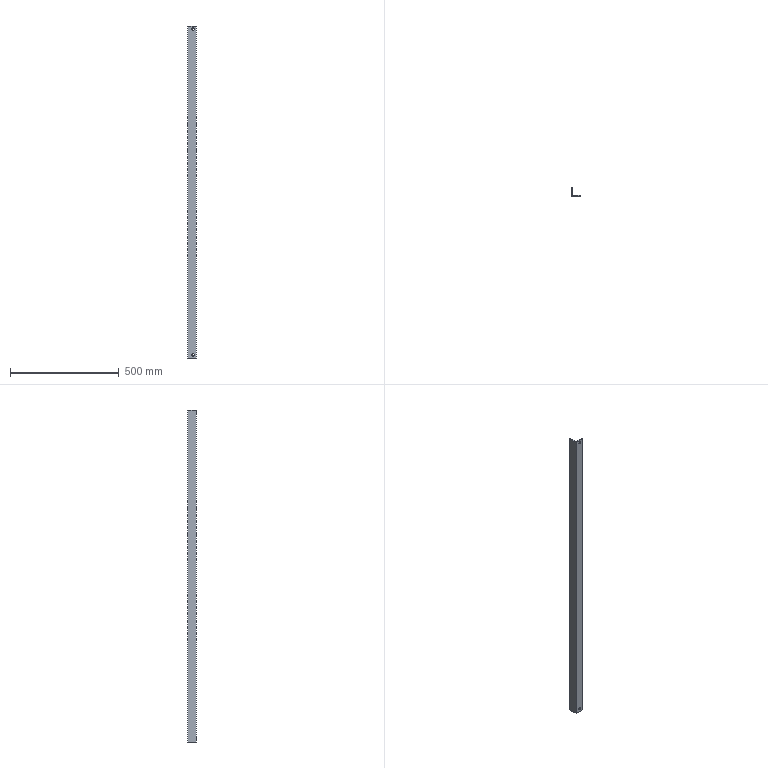Part | SolidWorks | features Cut 1, Extrusion 1 | 1 solid | 15 faces | box 40 x 40 x 1530 mm | volume 360303 mm3 | plane 8 | cylinder 7 | commonest cylinder face diameters 12 x4 2 x2 10 x1
STEP:
#1=CARTESIAN_POINT('',(25.,3.,1509.));
#2=VERTEX_POINT('',#1);
#3=CARTESIAN_POINT('',(25.,3.,1521.));
#4=VERTEX_POINT('',#3);
#5=CARTESIAN_POINT('',(25.,3.,1515.));
#6=DIRECTION('',(0.,1.,0.));
#7=DIRECTION('',(-1.,0.,0.));
#8=AXIS2_PLACEMENT_3D('',#5,#6,#7);
#9=CIRCLE('',#8,6.);
#10=EDGE_CURVE('',#2,#4,#9,.T.);
#11=ORIENTED_EDGE('',*,*,#10,.T.);
#12=CARTESIAN_POINT('',(25.,0.,1521.));
#13=VERTEX_POINT('',#12);
#14=CARTESIAN_POINT('',(25.,40.,1521.));
#15=DIRECTION('',(0.,-1.,0.));
#16=VECTOR('',#15,1000.);
#17=LINE('',#14,#16);
#18=EDGE_CURVE('',#4,#13,#17,.T.);
#19=ORIENTED_EDGE('',*,*,#18,.T.);
#20=CARTESIAN_POINT('',(25.,0.,1509.));
#21=VERTEX_POINT('',#20);
#22=CARTESIAN_POINT('',(25.,0.,1515.));
#23=DIRECTION('',(0.,-1.,0.));
#24=DIRECTION('',(0.,0.,-1.));
#25=AXIS2_PLACEMENT_3D('',#22,#23,#24);
#26=CIRCLE('',#25,6.);
#27=EDGE_CURVE('',#13,#21,#26,.T.);
#28=ORIENTED_EDGE('',*,*,#27,.T.);
#29=CARTESIAN_POINT('',(25.,40.,1509.));
#30=DIRECTION('',(0.,-1.,0.));
#31=VECTOR('',#30,1000.);
#32=LINE('',#29,#31);
#33=EDGE_CURVE('',#2,#21,#32,.T.);
#34=ORIENTED_EDGE('',*,*,#33,.F.);
#35=EDGE_LOOP('',(#11,#19,#28,#34));
#36=FACE_OUTER_BOUND('',#35,.T.);
#37=CARTESIAN_POINT('',(25.,40.,1515.));
#38=DIRECTION('',(0.,-1.,0.));
#39=DIRECTION('',(0.,0.,-1.));
#40=AXIS2_PLACEMENT_3D('',#37,#38,#39);
#41=CYLINDRICAL_SURFACE('',#40,6.);
#42=ADVANCED_FACE('',(#36),#41,.F.);
#43=CARTESIAN_POINT('',(25.,3.,9.));
#44=VERTEX_POINT('',#43);
#45=CARTESIAN_POINT('',(25.,3.,21.));
#46=VERTEX_POINT('',#45);
#47=CARTESIAN_POINT('',(25.,3.,15.));
#48=DIRECTION('',(0.,1.,0.));
#49=DIRECTION('',(-1.,0.,0.));
#50=AXIS2_PLACEMENT_3D('',#47,#48,#49);
#51=CIRCLE('',#50,6.);
#52=EDGE_CURVE('',#44,#46,#51,.T.);
#53=ORIENTED_EDGE('',*,*,#52,.T.);
#54=CARTESIAN_POINT('',(25.,0.,21.));
#55=VERTEX_POINT('',#54);
#56=CARTESIAN_POINT('',(25.,40.,21.));
#57=DIRECTION('',(0.,-1.,0.));
#58=VECTOR('',#57,1000.);
#59=LINE('',#56,#58);
#60=EDGE_CURVE('',#46,#55,#59,.T.);
#61=ORIENTED_EDGE('',*,*,#60,.T.);
#62=CARTESIAN_POINT('',(25.,0.,9.));
#63=VERTEX_POINT('',#62);
#64=CARTESIAN_POINT('',(25.,0.,15.));
#65=DIRECTION('',(0.,-1.,0.));
#66=DIRECTION('',(0.,0.,-1.));
#67=AXIS2_PLACEMENT_3D('',#64,#65,#66);
#68=CIRCLE('',#67,6.);
#69=EDGE_CURVE('',#55,#63,#68,.T.);
#70=ORIENTED_EDGE('',*,*,#69,.T.);
#71=CARTESIAN_POINT('',(25.,40.,9.));
#72=DIRECTION('',(0.,-1.,0.));
#73=VECTOR('',#72,1000.);
#74=LINE('',#71,#73);
#75=EDGE_CURVE('',#44,#63,#74,.T.);
#76=ORIENTED_EDGE('',*,*,#75,.F.);
#77=EDGE_LOOP('',(#53,#61,#70,#76));
#78=FACE_OUTER_BOUND('',#77,.T.);
#79=CARTESIAN_POINT('',(25.,40.,15.));
#80=DIRECTION('',(0.,-1.,0.));
#81=DIRECTION('',(0.,0.,-1.));
#82=AXIS2_PLACEMENT_3D('',#79,#80,#81);
#83=CYLINDRICAL_SURFACE('',#82,6.);
#84=ADVANCED_FACE('',(#78),#83,.F.);
#85=CARTESIAN_POINT('',(40.,0.,0.));
#86=VERTEX_POINT('',#85);
#87=CARTESIAN_POINT('',(40.,2.,0.));
#88=VERTEX_POINT('',#87);
#89=CARTESIAN_POINT('',(40.,0.,0.));
#90=DIRECTION('',(0.,1.,0.));
#91=VECTOR('',#90,1000.);
#92=LINE('',#89,#91);
#93=EDGE_CURVE('',#86,#88,#92,.T.);
#94=ORIENTED_EDGE('',*,*,#93,.T.);
#95=CARTESIAN_POINT('',(40.,2.,1530.));
#96=VERTEX_POINT('',#95);
#97=CARTESIAN_POINT('',(40.,2.,1530.));
#98=DIRECTION('',(0.,0.,-1.));
#99=VECTOR('',#98,1000.);
#100=LINE('',#97,#99);
#101=EDGE_CURVE('',#96,#88,#100,.T.);
#102=ORIENTED_EDGE('',*,*,#101,.F.);
#103=CARTESIAN_POINT('',(40.,0.,1530.));
#104=VERTEX_POINT('',#103);
#105=CARTESIAN_POINT('',(40.,0.,1530.));
#106=DIRECTION('',(0.,1.,0.));
#107=VECTOR('',#106,1000.);
#108=LINE('',#105,#107);
#109=EDGE_CURVE('',#104,#96,#108,.T.);
#110=ORIENTED_EDGE('',*,*,#109,.F.);
#111=CARTESIAN_POINT('',(40.,0.,1530.));
#112=DIRECTION('',(0.,0.,-1.));
#113=VECTOR('',#112,1000.);
#114=LINE('',#111,#113);
#115=EDGE_CURVE('',#104,#86,#114,.T.);
#116=ORIENTED_EDGE('',*,*,#115,.T.);
#117=EDGE_LOOP('',(#94,#102,#110,#116));
#118=FACE_OUTER_BOUND('',#117,.T.);
#119=CARTESIAN_POINT('',(40.,0.,1530.));
#120=DIRECTION('',(-1.,0.,0.));
#121=DIRECTION('',(0.,0.,1.));
#122=AXIS2_PLACEMENT_3D('',#119,#120,#121);
#123=PLANE('',#122);
#124=ADVANCED_FACE('',(#118),#123,.F.);
#125=CARTESIAN_POINT('',(39.,3.,0.));
#126=VERTEX_POINT('',#125);
#127=CARTESIAN_POINT('',(39.,2.,0.));
#128=DIRECTION('',(0.,0.,1.));
#129=DIRECTION('',(1.,0.,0.));
#130=AXIS2_PLACEMENT_3D('',#127,#128,#129);
#131=CIRCLE('',#130,1.);
#132=EDGE_CURVE('',#88,#126,#131,.T.);
#133=ORIENTED_EDGE('',*,*,#132,.T.);
#134=CARTESIAN_POINT('',(39.,3.,1530.));
#135=VERTEX_POINT('',#134);
#136=CARTESIAN_POINT('',(39.,3.,1530.));
#137=DIRECTION('',(0.,0.,-1.));
#138=VECTOR('',#137,1000.);
#139=LINE('',#136,#138);
#140=EDGE_CURVE('',#135,#126,#139,.T.);
#141=ORIENTED_EDGE('',*,*,#140,.F.);
#142=CARTESIAN_POINT('',(39.,2.,1530.));
#143=DIRECTION('',(0.,0.,1.));
#144=DIRECTION('',(1.,0.,0.));
#145=AXIS2_PLACEMENT_3D('',#142,#143,#144);
#146=CIRCLE('',#145,1.);
#147=EDGE_CURVE('',#96,#135,#146,.T.);
#148=ORIENTED_EDGE('',*,*,#147,.F.);
#149=ORIENTED_EDGE('',*,*,#101,.T.);
#150=EDGE_LOOP('',(#133,#141,#148,#149));
#151=FACE_OUTER_BOUND('',#150,.T.);
#152=CARTESIAN_POINT('',(39.,2.,1530.));
#153=DIRECTION('',(0.,0.,-1.));
#154=DIRECTION('',(-1.,0.,0.));
#155=AXIS2_PLACEMENT_3D('',#152,#153,#154);
#156=CYLINDRICAL_SURFACE('',#155,1.);
#157=ADVANCED_FACE('',(#151),#156,.T.);
#158=ORIENTED_EDGE('',*,*,#10,.F.);
#159=CARTESIAN_POINT('',(25.,3.,1515.));
#160=DIRECTION('',(0.,1.,0.));
#161=DIRECTION('',(-1.,0.,0.));
#162=AXIS2_PLACEMENT_3D('',#159,#160,#161);
#163=CIRCLE('',#162,6.);
#164=EDGE_CURVE('',#4,#2,#163,.T.);
#165=ORIENTED_EDGE('',*,*,#164,.F.);
#166=EDGE_LOOP('',(#158,#165));
#167=FACE_BOUND('',#166,.T.);
#168=ORIENTED_EDGE('',*,*,#52,.F.);
#169=CARTESIAN_POINT('',(25.,3.,15.));
#170=DIRECTION('',(0.,1.,0.));
#171=DIRECTION('',(-1.,0.,0.));
#172=AXIS2_PLACEMENT_3D('',#169,#170,#171);
#173=CIRCLE('',#172,6.);
#174=EDGE_CURVE('',#46,#44,#173,.T.);
#175=ORIENTED_EDGE('',*,*,#174,.F.);
#176=EDGE_LOOP('',(#168,#175));
#177=FACE_BOUND('',#176,.T.);
#178=CARTESIAN_POINT('',(8.,3.,0.));
#179=VERTEX_POINT('',#178);
#180=CARTESIAN_POINT('',(8.,3.,0.));
#181=DIRECTION('',(1.,0.,0.));
#182=VECTOR('',#181,1000.);
#183=LINE('',#180,#182);
#184=EDGE_CURVE('',#179,#126,#183,.T.);
#185=ORIENTED_EDGE('',*,*,#184,.F.);
#186=CARTESIAN_POINT('',(8.,3.,1530.));
#187=VERTEX_POINT('',#186);
#188=CARTESIAN_POINT('',(8.,3.,1530.));
#189=DIRECTION('',(0.,0.,-1.));
#190=VECTOR('',#189,1000.);
#191=LINE('',#188,#190);
#192=EDGE_CURVE('',#187,#179,#191,.T.);
#193=ORIENTED_EDGE('',*,*,#192,.F.);
#194=CARTESIAN_POINT('',(8.,3.,1530.));
#195=DIRECTION('',(1.,0.,0.));
#196=VECTOR('',#195,1000.);
#197=LINE('',#194,#196);
#198=EDGE_CURVE('',#187,#135,#197,.T.);
#199=ORIENTED_EDGE('',*,*,#198,.T.);
#200=ORIENTED_EDGE('',*,*,#140,.T.);
#201=EDGE_LOOP('',(#185,#193,#199,#200));
#202=FACE_OUTER_BOUND('',#201,.T.);
#203=CARTESIAN_POINT('',(8.,3.,1530.));
#204=DIRECTION('',(0.,1.,0.));
#205=DIRECTION('',(-1.,0.,0.));
#206=AXIS2_PLACEMENT_3D('',#203,#204,#205);
#207=PLANE('',#206);
#208=ADVANCED_FACE('',(#167,#177,#202),#207,.T.);
#209=CARTESIAN_POINT('',(3.,8.,0.));
#210=VERTEX_POINT('',#209);
#211=CARTESIAN_POINT('',(8.,8.,0.));
#212=DIRECTION('',(0.,0.,-1.));
#213=DIRECTION('',(-1.,0.,0.));
#214=AXIS2_PLACEMENT_3D('',#211,#212,#213);
#215=CIRCLE('',#214,5.);
#216=EDGE_CURVE('',#179,#210,#215,.T.);
#217=ORIENTED_EDGE('',*,*,#216,.T.);
#218=CARTESIAN_POINT('',(3.,8.,1530.));
#219=VERTEX_POINT('',#218);
#220=CARTESIAN_POINT('',(3.,8.,1530.));
#221=DIRECTION('',(0.,0.,-1.));
#222=VECTOR('',#221,1000.);
#223=LINE('',#220,#222);
#224=EDGE_CURVE('',#219,#210,#223,.T.);
#225=ORIENTED_EDGE('',*,*,#224,.F.);
#226=CARTESIAN_POINT('',(8.,8.,1530.));
#227=DIRECTION('',(0.,0.,-1.));
#228=DIRECTION('',(-1.,0.,0.));
#229=AXIS2_PLACEMENT_3D('',#226,#227,#228);
#230=CIRCLE('',#229,5.);
#231=EDGE_CURVE('',#187,#219,#230,.T.);
#232=ORIENTED_EDGE('',*,*,#231,.F.);
#233=ORIENTED_EDGE('',*,*,#192,.T.);
#234=EDGE_LOOP('',(#217,#225,#232,#233));
#235=FACE_OUTER_BOUND('',#234,.T.);
#236=CARTESIAN_POINT('',(8.,8.,1530.));
#237=DIRECTION('',(0.,0.,-1.));
#238=DIRECTION('',(-1.,0.,0.));
#239=AXIS2_PLACEMENT_3D('',#236,#237,#238);
#240=CYLINDRICAL_SURFACE('',#239,5.);
#241=ADVANCED_FACE('',(#235),#240,.F.);
#242=CARTESIAN_POINT('',(3.,39.,0.));
#243=VERTEX_POINT('',#242);
#244=CARTESIAN_POINT('',(3.,39.,0.));
#245=DIRECTION('',(0.,-1.,0.));
#246=VECTOR('',#245,1000.);
#247=LINE('',#244,#246);
#248=EDGE_CURVE('',#243,#210,#247,.T.);
#249=ORIENTED_EDGE('',*,*,#248,.F.);
#250=CARTESIAN_POINT('',(3.,39.,1530.));
#251=VERTEX_POINT('',#250);
#252=CARTESIAN_POINT('',(3.,39.,1530.));
#253=DIRECTION('',(0.,0.,-1.));
#254=VECTOR('',#253,1000.);
#255=LINE('',#252,#254);
#256=EDGE_CURVE('',#251,#243,#255,.T.);
#257=ORIENTED_EDGE('',*,*,#256,.F.);
#258=CARTESIAN_POINT('',(3.,39.,1530.));
#259=DIRECTION('',(0.,-1.,0.));
#260=VECTOR('',#259,1000.);
#261=LINE('',#258,#260);
#262=EDGE_CURVE('',#251,#219,#261,.T.);
#263=ORIENTED_EDGE('',*,*,#262,.T.);
#264=ORIENTED_EDGE('',*,*,#224,.T.);
#265=EDGE_LOOP('',(#249,#257,#263,#264));
#266=FACE_OUTER_BOUND('',#265,.T.);
#267=CARTESIAN_POINT('',(3.,39.,1530.));
#268=DIRECTION('',(1.,0.,0.));
#269=DIRECTION('',(0.,1.,0.));
#270=AXIS2_PLACEMENT_3D('',#267,#268,#269);
#271=PLANE('',#270);
#272=ADVANCED_FACE('',(#266),#271,.T.);
#273=CARTESIAN_POINT('',(2.,40.,0.));
#274=VERTEX_POINT('',#273);
#275=CARTESIAN_POINT('',(2.,39.,0.));
#276=DIRECTION('',(0.,0.,-1.));
#277=DIRECTION('',(-1.,0.,0.));
#278=AXIS2_PLACEMENT_3D('',#275,#276,#277);
#279=CIRCLE('',#278,1.);
#280=EDGE_CURVE('',#274,#243,#279,.T.);
#281=ORIENTED_EDGE('',*,*,#280,.F.);
#282=CARTESIAN_POINT('',(2.,40.,1530.));
#283=VERTEX_POINT('',#282);
#284=CARTESIAN_POINT('',(2.,40.,1530.));
#285=DIRECTION('',(0.,0.,-1.));
#286=VECTOR('',#285,1000.);
#287=LINE('',#284,#286);
#288=EDGE_CURVE('',#283,#274,#287,.T.);
#289=ORIENTED_EDGE('',*,*,#288,.F.);
#290=CARTESIAN_POINT('',(2.,39.,1530.));
#291=DIRECTION('',(0.,0.,-1.));
#292=DIRECTION('',(-1.,0.,0.));
#293=AXIS2_PLACEMENT_3D('',#290,#291,#292);
#294=CIRCLE('',#293,1.);
#295=EDGE_CURVE('',#283,#251,#294,.T.);
#296=ORIENTED_EDGE('',*,*,#295,.T.);
#297=ORIENTED_EDGE('',*,*,#256,.T.);
#298=EDGE_LOOP('',(#281,#289,#296,#297));
#299=FACE_OUTER_BOUND('',#298,.T.);
#300=CARTESIAN_POINT('',(2.,39.,1530.));
#301=DIRECTION('',(0.,0.,-1.));
#302=DIRECTION('',(-1.,0.,0.));
#303=AXIS2_PLACEMENT_3D('',#300,#301,#302);
#304=CYLINDRICAL_SURFACE('',#303,1.);
#305=ADVANCED_FACE('',(#299),#304,.T.);
#306=CARTESIAN_POINT('',(0.,40.,0.));
#307=VERTEX_POINT('',#306);
#308=CARTESIAN_POINT('',(0.,40.,0.));
#309=DIRECTION('',(1.,0.,0.));
#310=VECTOR('',#309,1000.);
#311=LINE('',#308,#310);
#312=EDGE_CURVE('',#307,#274,#311,.T.);
#313=ORIENTED_EDGE('',*,*,#312,.F.);
#314=CARTESIAN_POINT('',(0.,40.,1530.));
#315=VERTEX_POINT('',#314);
#316=CARTESIAN_POINT('',(0.,40.,1530.));
#317=DIRECTION('',(0.,0.,-1.));
#318=VECTOR('',#317,1000.);
#319=LINE('',#316,#318);
#320=EDGE_CURVE('',#315,#307,#319,.T.);
#321=ORIENTED_EDGE('',*,*,#320,.F.);
#322=CARTESIAN_POINT('',(0.,40.,1530.));
#323=DIRECTION('',(1.,0.,0.));
#324=VECTOR('',#323,1000.);
#325=LINE('',#322,#324);
#326=EDGE_CURVE('',#315,#283,#325,.T.);
#327=ORIENTED_EDGE('',*,*,#326,.T.);
#328=ORIENTED_EDGE('',*,*,#288,.T.);
#329=EDGE_LOOP('',(#313,#321,#327,#328));
#330=FACE_OUTER_BOUND('',#329,.T.);
#331=CARTESIAN_POINT('',(0.,40.,1530.));
#332=DIRECTION('',(0.,1.,0.));
#333=DIRECTION('',(0.,0.,1.));
#334=AXIS2_PLACEMENT_3D('',#331,#332,#333);
#335=PLANE('',#334);
#336=ADVANCED_FACE('',(#330),#335,.T.);
#337=CARTESIAN_POINT('',(0.,0.,0.));
#338=VERTEX_POINT('',#337);
#339=CARTESIAN_POINT('',(0.,0.,0.));
#340=DIRECTION('',(0.,1.,0.));
#341=VECTOR('',#340,1000.);
#342=LINE('',#339,#341);
#343=EDGE_CURVE('',#338,#307,#342,.T.);
#344=ORIENTED_EDGE('',*,*,#343,.F.);
#345=CARTESIAN_POINT('',(0.,0.,1530.));
#346=VERTEX_POINT('',#345);
#347=CARTESIAN_POINT('',(0.,0.,1530.));
#348=DIRECTION('',(0.,0.,-1.));
#349=VECTOR('',#348,1000.);
#350=LINE('',#347,#349);
#351=EDGE_CURVE('',#346,#338,#350,.T.);
#352=ORIENTED_EDGE('',*,*,#351,.F.);
#353=CARTESIAN_POINT('',(0.,0.,1530.));
#354=DIRECTION('',(0.,1.,0.));
#355=VECTOR('',#354,1000.);
#356=LINE('',#353,#355);
#357=EDGE_CURVE('',#346,#315,#356,.T.);
#358=ORIENTED_EDGE('',*,*,#357,.T.);
#359=ORIENTED_EDGE('',*,*,#320,.T.);
#360=EDGE_LOOP('',(#344,#352,#358,#359));
#361=FACE_OUTER_BOUND('',#360,.T.);
#362=CARTESIAN_POINT('',(0.,0.,1530.));
#363=DIRECTION('',(-1.,0.,0.));
#364=DIRECTION('',(0.,0.,1.));
#365=AXIS2_PLACEMENT_3D('',#362,#363,#364);
#366=PLANE('',#365);
#367=ADVANCED_FACE('',(#361),#366,.T.);
#368=CARTESIAN_POINT('',(25.,0.,1515.));
#369=DIRECTION('',(0.,-1.,0.));
#370=DIRECTION('',(0.,0.,-1.));
#371=AXIS2_PLACEMENT_3D('',#368,#369,#370);
#372=CIRCLE('',#371,6.);
#373=EDGE_CURVE('',#21,#13,#372,.T.);
#374=ORIENTED_EDGE('',*,*,#373,.F.);
#375=ORIENTED_EDGE('',*,*,#27,.F.);
#376=EDGE_LOOP('',(#374,#375));
#377=FACE_BOUND('',#376,.T.);
#378=CARTESIAN_POINT('',(25.,0.,15.));
#379=DIRECTION('',(0.,-1.,0.));
#380=DIRECTION('',(0.,0.,-1.));
#381=AXIS2_PLACEMENT_3D('',#378,#379,#380);
#382=CIRCLE('',#381,6.);
#383=EDGE_CURVE('',#63,#55,#382,.T.);
#384=ORIENTED_EDGE('',*,*,#383,.F.);
#385=ORIENTED_EDGE('',*,*,#69,.F.);
#386=EDGE_LOOP('',(#384,#385));
#387=FACE_BOUND('',#386,.T.);
#388=CARTESIAN_POINT('',(40.,0.,0.));
#389=DIRECTION('',(-1.,0.,0.));
#390=VECTOR('',#389,1000.);
#391=LINE('',#388,#390);
#392=EDGE_CURVE('',#86,#338,#391,.T.);
#393=ORIENTED_EDGE('',*,*,#392,.F.);
#394=ORIENTED_EDGE('',*,*,#115,.F.);
#395=CARTESIAN_POINT('',(40.,0.,1530.));
#396=DIRECTION('',(-1.,0.,0.));
#397=VECTOR('',#396,1000.);
#398=LINE('',#395,#397);
#399=EDGE_CURVE('',#104,#346,#398,.T.);
#400=ORIENTED_EDGE('',*,*,#399,.T.);
#401=ORIENTED_EDGE('',*,*,#351,.T.);
#402=EDGE_LOOP('',(#393,#394,#400,#401));
#403=FACE_OUTER_BOUND('',#402,.T.);
#404=CARTESIAN_POINT('',(40.,0.,1530.));
#405=DIRECTION('',(0.,-1.,0.));
#406=DIRECTION('',(0.,0.,-1.));
#407=AXIS2_PLACEMENT_3D('',#404,#405,#406);
#408=PLANE('',#407);
#409=ADVANCED_FACE('',(#377,#387,#403),#408,.T.);
#410=ORIENTED_EDGE('',*,*,#109,.T.);
#411=ORIENTED_EDGE('',*,*,#147,.T.);
#412=ORIENTED_EDGE('',*,*,#198,.F.);
#413=ORIENTED_EDGE('',*,*,#231,.T.);
#414=ORIENTED_EDGE('',*,*,#262,.F.);
#415=ORIENTED_EDGE('',*,*,#295,.F.);
#416=ORIENTED_EDGE('',*,*,#326,.F.);
#417=ORIENTED_EDGE('',*,*,#357,.F.);
#418=ORIENTED_EDGE('',*,*,#399,.F.);
#419=EDGE_LOOP('',(#410,#411,#412,#413,#414,#415,#416,#417,#418));
#420=FACE_OUTER_BOUND('',#419,.T.);
#421=CARTESIAN_POINT('',(39.,2.,1530.));
#422=DIRECTION('',(0.,0.,1.));
#423=DIRECTION('',(1.,0.,0.));
#424=AXIS2_PLACEMENT_3D('',#421,#422,#423);
#425=PLANE('',#424);
#426=ADVANCED_FACE('',(#420),#425,.T.);
#427=ORIENTED_EDGE('',*,*,#93,.F.);
#428=ORIENTED_EDGE('',*,*,#392,.T.);
#429=ORIENTED_EDGE('',*,*,#343,.T.);
#430=ORIENTED_EDGE('',*,*,#312,.T.);
#431=ORIENTED_EDGE('',*,*,#280,.T.);
#432=ORIENTED_EDGE('',*,*,#248,.T.);
#433=ORIENTED_EDGE('',*,*,#216,.F.);
#434=ORIENTED_EDGE('',*,*,#184,.T.);
#435=ORIENTED_EDGE('',*,*,#132,.F.);
#436=EDGE_LOOP('',(#427,#428,#429,#430,#431,#432,#433,#434,#435));
#437=FACE_OUTER_BOUND('',#436,.T.);
#438=CARTESIAN_POINT('',(39.,2.,0.));
#439=DIRECTION('',(0.,0.,1.));
#440=DIRECTION('',(1.,0.,0.));
#441=AXIS2_PLACEMENT_3D('',#438,#439,#440);
#442=PLANE('',#441);
#443=ADVANCED_FACE('',(#437),#442,.F.);
#444=ORIENTED_EDGE('',*,*,#60,.F.);
#445=ORIENTED_EDGE('',*,*,#174,.T.);
#446=ORIENTED_EDGE('',*,*,#75,.T.);
#447=ORIENTED_EDGE('',*,*,#383,.T.);
#448=EDGE_LOOP('',(#444,#445,#446,#447));
#449=FACE_OUTER_BOUND('',#448,.T.);
#450=CARTESIAN_POINT('',(25.,40.,15.));
#451=DIRECTION('',(0.,-1.,0.));
#452=DIRECTION('',(0.,0.,-1.));
#453=AXIS2_PLACEMENT_3D('',#450,#451,#452);
#454=CYLINDRICAL_SURFACE('',#453,6.);
#455=ADVANCED_FACE('',(#449),#454,.F.);
#456=ORIENTED_EDGE('',*,*,#18,.F.);
#457=ORIENTED_EDGE('',*,*,#164,.T.);
#458=ORIENTED_EDGE('',*,*,#33,.T.);
#459=ORIENTED_EDGE('',*,*,#373,.T.);
#460=EDGE_LOOP('',(#456,#457,#458,#459));
#461=FACE_OUTER_BOUND('',#460,.T.);
#462=CARTESIAN_POINT('',(25.,40.,1515.));
#463=DIRECTION('',(0.,-1.,0.));
#464=DIRECTION('',(0.,0.,-1.));
#465=AXIS2_PLACEMENT_3D('',#462,#463,#464);
#466=CYLINDRICAL_SURFACE('',#465,6.);
#467=ADVANCED_FACE('',(#461),#466,.F.);
#468=CLOSED_SHELL('',(#42,#84,#124,#157,#208,#241,#272,#305,#336,#367,#409,#426,#443,#455,#467));
#469=MANIFOLD_SOLID_BREP('',#468);
#470=CARTESIAN_POINT('',(0.,0.,0.));
#471=DIRECTION('',(0.,0.,1.));
#472=DIRECTION('',(1.,0.,0.));
#473=AXIS2_PLACEMENT_3D('',#470,#471,#472);
#474=(LENGTH_UNIT()NAMED_UNIT(*)SI_UNIT(.MILLI.,.METRE.));
#475=UNCERTAINTY_MEASURE_WITH_UNIT(LENGTH_MEASURE(0.00001),#474,'','');
#476=(NAMED_UNIT(*)PLANE_ANGLE_UNIT()SI_UNIT($,.RADIAN.));
#477=(NAMED_UNIT(*)SI_UNIT($,.STERADIAN.)SOLID_ANGLE_UNIT());
#478=(GEOMETRIC_REPRESENTATION_CONTEXT(3)GLOBAL_UNCERTAINTY_ASSIGNED_CONTEXT((#475))GLOBAL_UNIT_ASSIGNED_CONTEXT((#474,#476,#477))REPRESENTATION_CONTEXT('',''));
#479=ADVANCED_BREP_SHAPE_REPRESENTATION('',(#469,#473),#478);